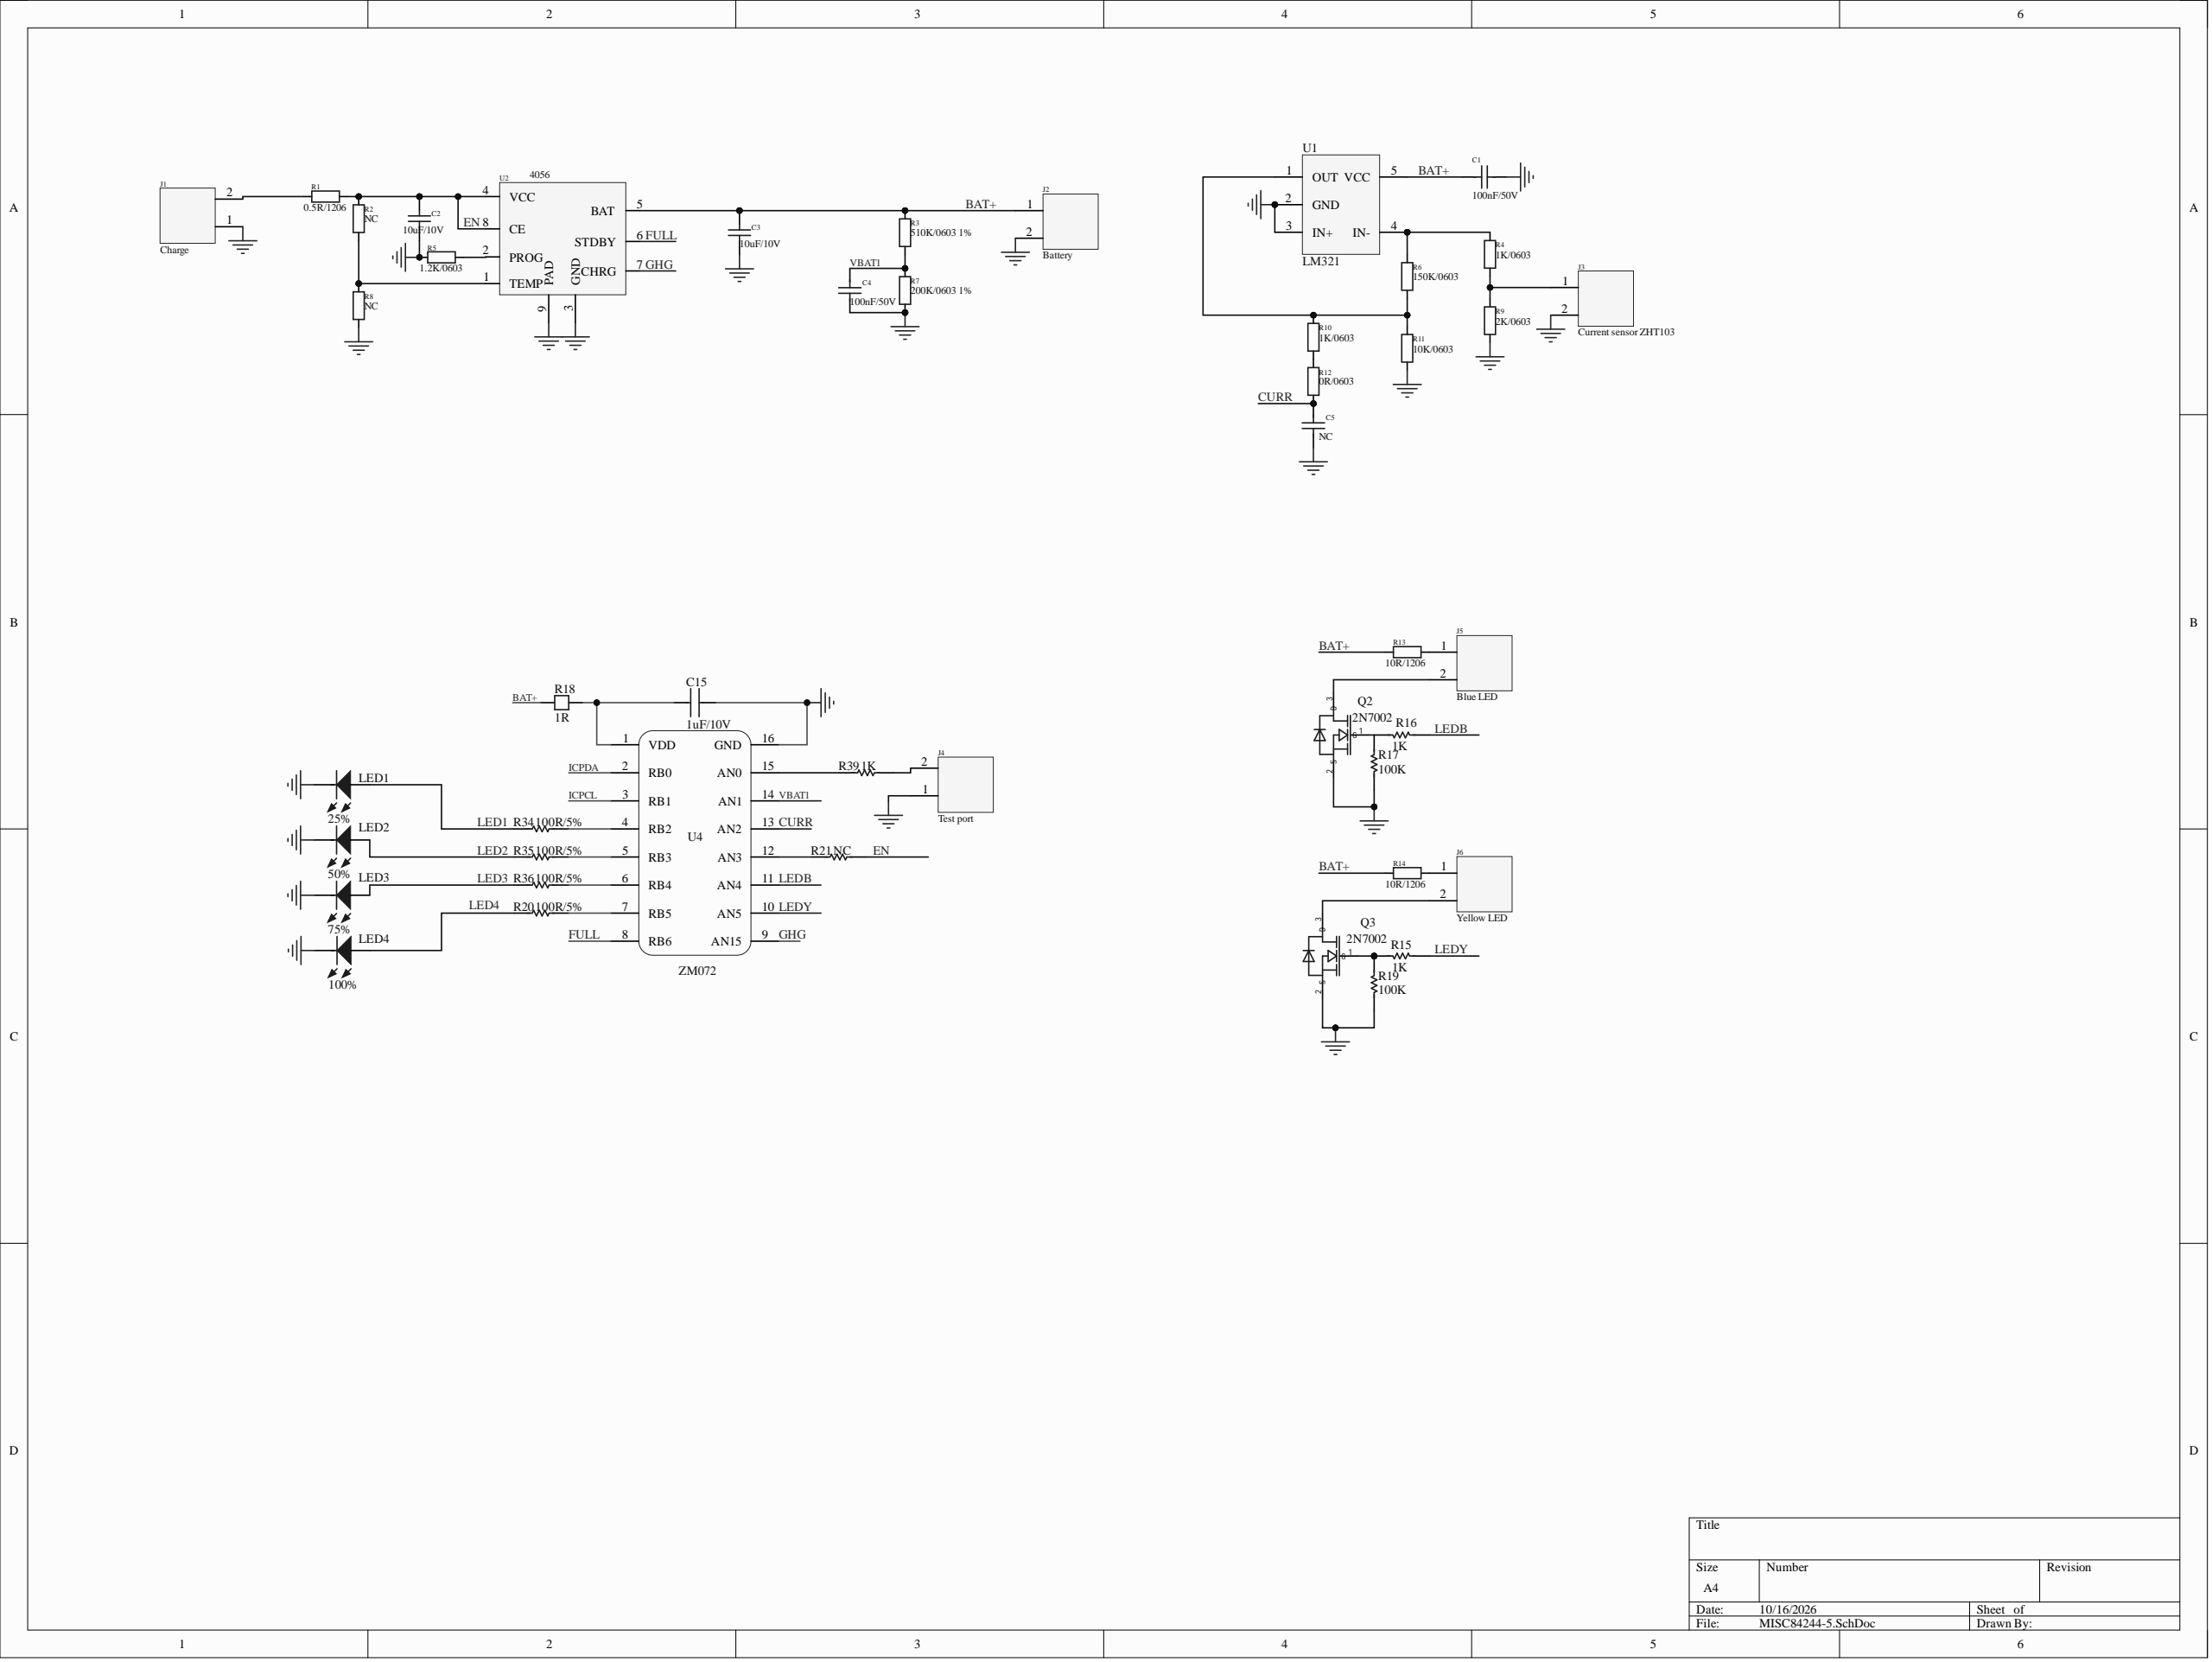Circuit board | Altium Designer | 46 parts | 34 nets
Bill of materials:
Comment,Description,Designator,Footprint,LibRef,Quantity
"100nF/50V","","C1, C4","C0603A","Cap0603","2"
"10uF/10V","SMD capacitor","C2, C3","C0805A","Cap0805","2"
"NC","","C5","C0603A","Cap0603","1"
"1uF/10V","","C15","C0603A","CH","1"
"Charge","DC jack right-angle 90° pitch 2.0","J1","HY2.0WT-2A/P 立贴带扣耐温260℃","2PIN","1"
"Battery","DC jack right-angle 90° pitch 2.0","J2","GH1.25-2PIN立贴带扣耐温260℃","2PIN","1"
"Current sensor ZHT103","DC jack right-angle 90° pitch 2.0","J3","IND-TH_L18.2-W10.2-P12.00-D0.9_ZHT103","2PIN","1"
"Test port","DC jack right-angle 90° pitch 2.0","J4","HY2.0WT-2A/P 立贴带扣耐温260℃","2PIN","1"
"Blue LED","DC jack right-angle 90° pitch 2.0","J5","GH1.25-2PIN立贴带扣耐温260℃","2PIN","1"
"Yellow LED","DC jack right-angle 90° pitch 2.0","J6","GH1.25-2PIN立贴带扣耐温260℃","2PIN","1"
"25%","SMD LED","LED1","LED0603A","LED 白发蓝","1"
"50%","SMD LED","LED2","LED0603A","LED 白发蓝","1"
"75%","SMD LED","LED3","LED0603A","LED 白发蓝","1"
"100%","SMD LED","LED4","LED0603A","LED 白发蓝","1"
"2N7002","SMD MOSFET","Q2, Q3","SOT23-3L","2N7002","2"
"0.5R/1206","SMD resistor","R1","R1206A","Res1206","1"
"NC","SMD resistor","R2, R8, R21","R0603A","Res0603","3"
"510K/0603 1%","SMD resistor","R3","R0603A","Res0603","1"
"1K/0603","SMD resistor","R4, R10","R0603A","Res0603","2"
"1.2K/0603","SMD resistor","R5","R0603A","Res0603","1"
"150K/0603","SMD resistor","R6","R0603A","Res0603","1"
"200K/0603 1%","SMD resistor","R7","R0603A","Res0603","1"
"2K/0603","SMD resistor","R9","R0603A","Res0603","1"
"10K/0603","SMD resistor","R11","R0603A","Res0603","1"
"0R/0603","SMD resistor","R12","R0603A","Res0603","1"
"10R/1206","SMD resistor","R13, R14","R1206A","Res1206","2"
"1K","SMD resistor","R15, R16, R39","R0603A","Res0603","3"
"100K","SMD resistor","R17, R19","R0603A","Res0603","2"
"1R","","R18","R0603A","RH1","1"
"100R/5%","SMD resistor","R20, R34, R35, R36","R0603A","Res0603","4"
"LM321","","U1","SOT23-5A","LM321","1"
"4056","Charger IC","U2","ESOP-8L","TP4056","1"
"ZM072","","U4","SOP16L","MCU-TSSOP-16","1"
Netlist (Protel format):
[
C1
C0603A
100nF/50V



]
[
C2
C0805A
10uF/10V



]
[
C3
C0805A
10uF/10V



]
[
C4
C0603A
100nF/50V



]
[
C5
C0603A
NC



]
[
C15
C0603A
1uF/10V



]
[
J1
HY2.0WT-2A/P 立贴带扣耐温260℃
Charge



]
[
J2
GH1.25-2PIN立贴带扣耐温260℃
Battery



]
[
J3
IND-TH_L18.2-W10.2-P12.00-D0.9_ZHT103
Current sensor ZHT103



]
[
J4
HY2.0WT-2A/P 立贴带扣耐温260℃
Test port



]
[
J5
GH1.25-2PIN立贴带扣耐温260℃
Blue LED



]
[
J6
GH1.25-2PIN立贴带扣耐温260℃
Yellow LED



]
[
LED1
LED0603A
25%



]
[
LED2
LED0603A
50%



]
[
LED3
LED0603A
75%



]
[
LED4
LED0603A
100%



]
[
Q2
SOT23-3L
2N7002



]
[
Q3
SOT23-3L
2N7002



]
[
R1
R1206A
0.5R/1206



]
[
R2
R0603A
NC



]
[
R3
R0603A
510K/0603 1%



]
[
R4
R0603A
1K/0603



]
[
R5
R0603A
1.2K/0603



]
[
R6
R0603A
150K/0603



]
[
R7
R0603A
200K/0603 1%



]
[
R8
R0603A
NC



]
[
R9
R0603A
2K/0603



]
[
R10
R0603A
1K/0603



]
[
R11
R0603A
10K/0603



]
[
R12
R0603A
0R/0603



]
[
R13
R1206A
10R/1206



]
[
R14
R1206A
10R/1206



]
[
R15
R0603A
1K



]
[
R16
R0603A
1K



]
[
R17
R0603A
100K



]
[
R18
R0603A
1R



]
[
R19
R0603A
100K



]
[
R20
R0603A
100R/5%



]
[
R21
R0603A
NC



]
[
R34
R0603A
100R/5%



]
[
R35
R0603A
100R/5%



]
[
R36
R0603A
100R/5%



]
[
R39
R0603A
1K



]
[
U1
SOT23-5A
LM321



]
[
U2
ESOP-8L
4056



]
[
U4
SOP16L
ZM072



]
(
VBAT1
C4-2
R3-1
R7-2
U4-14
)
(
NetR39_1
R39-1
U4-15
)
(
NetR36_2
R36-2
U4-6
)
(
NetR35_2
R35-2
U4-5
)
(
NetR34_2
R34-2
U4-4
)
(
NetR21_1
R21-1
U4-12
)
(
NetR20_2
R20-2
U4-7
)
(
NetR10_2
R10-2
R12-1
)
(
NetR6_2
R6-2
R10-1
R11-1
U1-1
)
(
NetR5_2
R5-2
U2-2
)
(
NetR4_1
R4-1
R6-1
U1-4
)
(
NetR2_1
R2-1
R8-2
U2-1
)
(
NetQ3_1
Q3-1
R15-1
R19-2
)
(
NetQ2_1
Q2-1
R16-1
R17-2
)
(
NetLED4_1
LED4-1
R20-1
)
(
NetJ6_2
J6-2
Q3-3
)
(
NetJ6_1
J6-1
R14-2
)
(
NetJ5_2
J5-2
Q2-3
)
(
NetJ5_1
J5-1
R13-2
)
(
NetJ4_2
J4-2
R39-2
)
(
NetJ3_1
J3-1
R4-2
R9-1
)
(
NetJ1_2
J1-2
R1-1
)
(
NetC15_1
C15-1
R18-2
U4-1
)
(
LEDY
R15-2
U4-10
)
(
LEDB
R16-2
U4-11
)
(
LED3
LED3-1
R36-1
)
(
LED2
LED2-1
R35-1
)
(
LED1
LED1-1
R34-1
)
(
GND
C1-1
C2-1
C3-1
C4-1
C5-1
C15-2
J1-1
J2-2
J3-2
J4-1
LED1-2
LED2-2
LED3-2
LED4-2
Q2-2
Q3-2
R5-1
R7-1
R8-1
R9-2
R11-2
R17-1
R19-1
U1-2
U1-3
U2-3
U2-9
U4-16
)
(
GHG
U2-7
U4-9
)
(
FULL
U2-6
U4-8
)
(
EN
C2-2
R1-2
R2-2
R21-2
U2-4
U2-8
)
(
CURR
C5-2
R12-2
U4-13
)
(
BAT+
C1-2
C3-2
J2-1
R3-2
R13-1
R14-1
R18-1
U1-5
U2-5
)